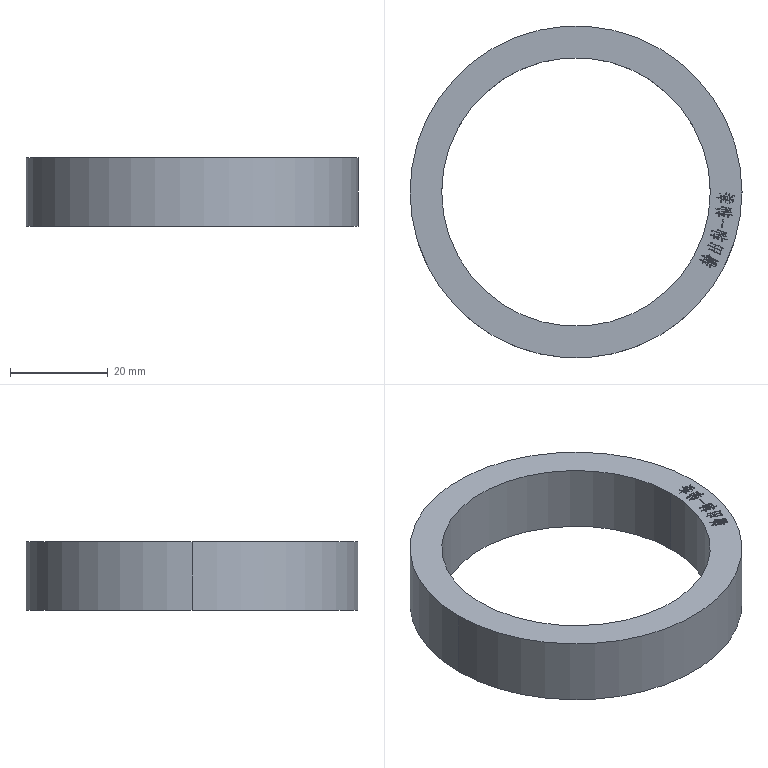Part | SolidWorks | features Extrusion 1, ICE 1 | 1 solid | 687 faces | box 68 x 68 x 14 mm | volume 17581 mm3 | plane 511 | spline 172 | cylinder 4 | commonest cylinder face diameters 55 x2 68 x2